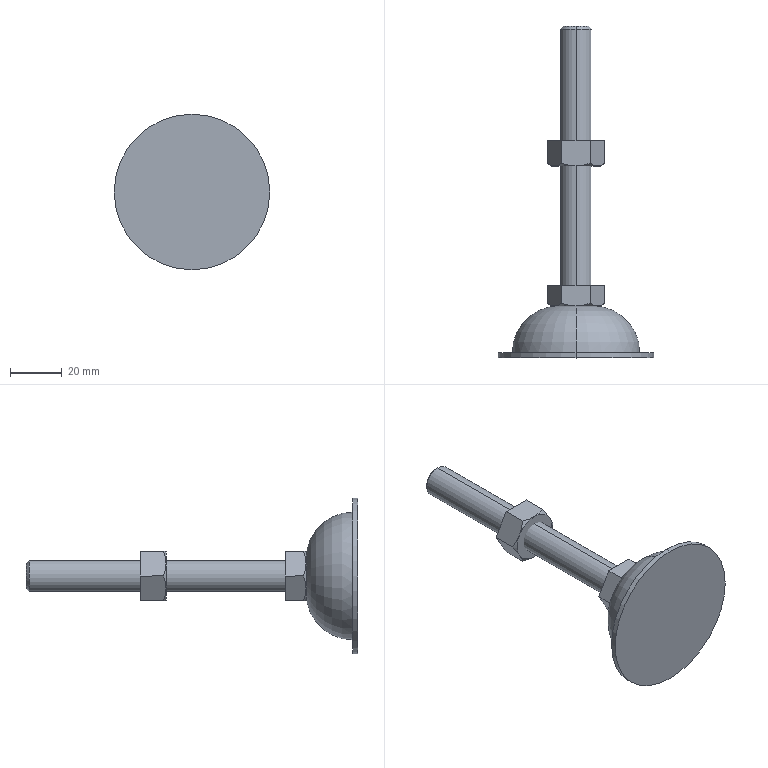Part | SolidWorks | features ICE 4, Chamfer 1, Revolution 1 | 2 solids | 39 faces | box 60 x 128 x 60 mm | volume 47779 mm3 | plane 19 | cone 14 | cylinder 4 | torus 2 | commonest cylinder face diameters 12 x2 60 x2
STEP:
#1=CARTESIAN_POINT('',(0.,28.,6.));
#2=VERTEX_POINT('',#1);
#3=CARTESIAN_POINT('',(0.,28.,-6.));
#4=VERTEX_POINT('',#3);
#5=CARTESIAN_POINT('',(0.,28.,0.));
#6=DIRECTION('',(0.,1.,0.));
#7=DIRECTION('',(0.,0.,1.));
#8=AXIS2_PLACEMENT_3D('',#5,#6,#7);
#9=CIRCLE('',#8,6.);
#10=EDGE_CURVE('',#2,#4,#9,.T.);
#11=ORIENTED_EDGE('',*,*,#10,.T.);
#12=CARTESIAN_POINT('',(0.,126.8,-6.));
#13=VERTEX_POINT('',#12);
#14=CARTESIAN_POINT('',(0.,128.,-6.));
#15=DIRECTION('',(0.,1.,0.));
#16=VECTOR('',#15,1000.);
#17=LINE('',#14,#16);
#18=EDGE_CURVE('',#4,#13,#17,.T.);
#19=ORIENTED_EDGE('',*,*,#18,.T.);
#20=CARTESIAN_POINT('',(0.,126.8,6.));
#21=VERTEX_POINT('',#20);
#22=CARTESIAN_POINT('',(0.,126.8,0.));
#23=DIRECTION('',(0.,-1.,0.));
#24=DIRECTION('',(0.,0.,-1.));
#25=AXIS2_PLACEMENT_3D('',#22,#23,#24);
#26=CIRCLE('',#25,6.);
#27=EDGE_CURVE('',#13,#21,#26,.T.);
#28=ORIENTED_EDGE('',*,*,#27,.T.);
#29=CARTESIAN_POINT('',(0.,128.,6.));
#30=DIRECTION('',(0.,1.,0.));
#31=VECTOR('',#30,1000.);
#32=LINE('',#29,#31);
#33=EDGE_CURVE('',#2,#21,#32,.T.);
#34=ORIENTED_EDGE('',*,*,#33,.F.);
#35=EDGE_LOOP('',(#11,#19,#28,#34));
#36=FACE_OUTER_BOUND('',#35,.T.);
#37=CARTESIAN_POINT('',(0.,128.,0.));
#38=DIRECTION('',(0.,1.,0.));
#39=DIRECTION('',(0.,0.,1.));
#40=AXIS2_PLACEMENT_3D('',#37,#38,#39);
#41=CYLINDRICAL_SURFACE('',#40,6.);
#42=ADVANCED_FACE('',(#36),#41,.T.);
#43=CARTESIAN_POINT('',(0.,128.,4.8));
#44=VERTEX_POINT('',#43);
#45=CARTESIAN_POINT('',(0.,128.,-4.8));
#46=VERTEX_POINT('',#45);
#47=CARTESIAN_POINT('',(0.,128.,0.));
#48=DIRECTION('',(0.,1.,0.));
#49=DIRECTION('',(0.,0.,-1.));
#50=AXIS2_PLACEMENT_3D('',#47,#48,#49);
#51=CIRCLE('',#50,4.8);
#52=EDGE_CURVE('',#44,#46,#51,.T.);
#53=ORIENTED_EDGE('',*,*,#52,.F.);
#54=CARTESIAN_POINT('',(0.,128.,4.8));
#55=DIRECTION('',(0.,-0.7071,0.7071));
#56=VECTOR('',#55,1000.);
#57=LINE('',#54,#56);
#58=EDGE_CURVE('',#44,#21,#57,.T.);
#59=ORIENTED_EDGE('',*,*,#58,.T.);
#60=ORIENTED_EDGE('',*,*,#27,.F.);
#61=CARTESIAN_POINT('',(0.,128.,-4.8));
#62=DIRECTION('',(0.,-0.7071,-0.7071));
#63=VECTOR('',#62,1000.);
#64=LINE('',#61,#63);
#65=EDGE_CURVE('',#46,#13,#64,.T.);
#66=ORIENTED_EDGE('',*,*,#65,.F.);
#67=EDGE_LOOP('',(#53,#59,#60,#66));
#68=FACE_OUTER_BOUND('',#67,.T.);
#69=CARTESIAN_POINT('',(0.,128.,0.));
#70=DIRECTION('',(0.,-1.,0.));
#71=DIRECTION('',(0.,0.,-1.));
#72=AXIS2_PLACEMENT_3D('',#69,#70,#71);
#73=CONICAL_SURFACE('',#72,4.8,0.7854);
#74=ADVANCED_FACE('',(#68),#73,.T.);
#75=CARTESIAN_POINT('',(0.,2.,24.6));
#76=VERTEX_POINT('',#75);
#77=CARTESIAN_POINT('',(0.,2.,-24.6));
#78=VERTEX_POINT('',#77);
#79=CARTESIAN_POINT('',(0.,2.,0.));
#80=DIRECTION('',(0.,1.,0.));
#81=DIRECTION('',(0.,0.,1.));
#82=AXIS2_PLACEMENT_3D('',#79,#80,#81);
#83=CIRCLE('',#82,24.6);
#84=EDGE_CURVE('',#76,#78,#83,.T.);
#85=ORIENTED_EDGE('',*,*,#84,.T.);
#86=CARTESIAN_POINT('',(0.,20.,-6.6));
#87=VERTEX_POINT('',#86);
#88=CARTESIAN_POINT('',(0.,2.,-6.6));
#89=DIRECTION('',(1.,0.,0.));
#90=DIRECTION('',(0.,0.,-1.));
#91=AXIS2_PLACEMENT_3D('',#88,#89,#90);
#92=CIRCLE('',#91,18.);
#93=EDGE_CURVE('',#78,#87,#92,.T.);
#94=ORIENTED_EDGE('',*,*,#93,.T.);
#95=CARTESIAN_POINT('',(0.,20.,6.6));
#96=VERTEX_POINT('',#95);
#97=CARTESIAN_POINT('',(0.,20.,0.));
#98=DIRECTION('',(0.,1.,0.));
#99=DIRECTION('',(0.,0.,1.));
#100=AXIS2_PLACEMENT_3D('',#97,#98,#99);
#101=CIRCLE('',#100,6.6);
#102=EDGE_CURVE('',#96,#87,#101,.T.);
#103=ORIENTED_EDGE('',*,*,#102,.F.);
#104=CARTESIAN_POINT('',(0.,2.,6.6));
#105=DIRECTION('',(-1.,0.,0.));
#106=DIRECTION('',(0.,0.,1.));
#107=AXIS2_PLACEMENT_3D('',#104,#105,#106);
#108=CIRCLE('',#107,18.);
#109=EDGE_CURVE('',#76,#96,#108,.T.);
#110=ORIENTED_EDGE('',*,*,#109,.F.);
#111=EDGE_LOOP('',(#85,#94,#103,#110));
#112=FACE_OUTER_BOUND('',#111,.T.);
#113=CARTESIAN_POINT('',(0.,2.,0.));
#114=DIRECTION('',(0.,1.,0.));
#115=DIRECTION('',(0.,0.,1.));
#116=AXIS2_PLACEMENT_3D('',#113,#114,#115);
#117=TOROIDAL_SURFACE('',#116,6.6,18.);
#118=ADVANCED_FACE('',(#112),#117,.T.);
#119=CARTESIAN_POINT('',(0.,0.,30.));
#120=VERTEX_POINT('',#119);
#121=CARTESIAN_POINT('',(0.,0.,-30.));
#122=VERTEX_POINT('',#121);
#123=CARTESIAN_POINT('',(0.,0.,0.));
#124=DIRECTION('',(0.,1.,0.));
#125=DIRECTION('',(0.,0.,1.));
#126=AXIS2_PLACEMENT_3D('',#123,#124,#125);
#127=CIRCLE('',#126,30.);
#128=EDGE_CURVE('',#120,#122,#127,.T.);
#129=ORIENTED_EDGE('',*,*,#128,.T.);
#130=CARTESIAN_POINT('',(0.,2.,-30.));
#131=VERTEX_POINT('',#130);
#132=CARTESIAN_POINT('',(0.,128.,-30.));
#133=DIRECTION('',(0.,1.,0.));
#134=VECTOR('',#133,1000.);
#135=LINE('',#132,#134);
#136=EDGE_CURVE('',#122,#131,#135,.T.);
#137=ORIENTED_EDGE('',*,*,#136,.T.);
#138=CARTESIAN_POINT('',(0.,2.,30.));
#139=VERTEX_POINT('',#138);
#140=CARTESIAN_POINT('',(0.,2.,0.));
#141=DIRECTION('',(0.,1.,0.));
#142=DIRECTION('',(0.,0.,1.));
#143=AXIS2_PLACEMENT_3D('',#140,#141,#142);
#144=CIRCLE('',#143,30.);
#145=EDGE_CURVE('',#139,#131,#144,.T.);
#146=ORIENTED_EDGE('',*,*,#145,.F.);
#147=CARTESIAN_POINT('',(0.,128.,30.));
#148=DIRECTION('',(0.,1.,0.));
#149=VECTOR('',#148,1000.);
#150=LINE('',#147,#149);
#151=EDGE_CURVE('',#120,#139,#150,.T.);
#152=ORIENTED_EDGE('',*,*,#151,.F.);
#153=EDGE_LOOP('',(#129,#137,#146,#152));
#154=FACE_OUTER_BOUND('',#153,.T.);
#155=CARTESIAN_POINT('',(0.,128.,0.));
#156=DIRECTION('',(0.,1.,0.));
#157=DIRECTION('',(0.,0.,1.));
#158=AXIS2_PLACEMENT_3D('',#155,#156,#157);
#159=CYLINDRICAL_SURFACE('',#158,30.);
#160=ADVANCED_FACE('',(#154),#159,.T.);
#161=ORIENTED_EDGE('',*,*,#102,.T.);
#162=CARTESIAN_POINT('',(0.,20.,0.));
#163=DIRECTION('',(0.,1.,0.));
#164=DIRECTION('',(0.,0.,1.));
#165=AXIS2_PLACEMENT_3D('',#162,#163,#164);
#166=CIRCLE('',#165,6.6);
#167=EDGE_CURVE('',#87,#96,#166,.T.);
#168=ORIENTED_EDGE('',*,*,#167,.T.);
#169=EDGE_LOOP('',(#161,#168));
#170=FACE_BOUND('',#169,.T.);
#171=CARTESIAN_POINT('',(8.227,20.,4.75));
#172=VERTEX_POINT('',#171);
#173=CARTESIAN_POINT('',(0.,20.,9.5));
#174=VERTEX_POINT('',#173);
#175=CARTESIAN_POINT('',(0.,20.,0.));
#176=DIRECTION('',(0.,-1.,0.));
#177=DIRECTION('',(0.,0.,-1.));
#178=AXIS2_PLACEMENT_3D('',#175,#176,#177);
#179=CIRCLE('',#178,9.5);
#180=EDGE_CURVE('',#172,#174,#179,.T.);
#181=ORIENTED_EDGE('',*,*,#180,.T.);
#182=CARTESIAN_POINT('',(-8.227,20.,4.75));
#183=VERTEX_POINT('',#182);
#184=CARTESIAN_POINT('',(0.,20.,0.));
#185=DIRECTION('',(0.,-1.,0.));
#186=DIRECTION('',(0.,0.,-1.));
#187=AXIS2_PLACEMENT_3D('',#184,#185,#186);
#188=CIRCLE('',#187,9.5);
#189=EDGE_CURVE('',#174,#183,#188,.T.);
#190=ORIENTED_EDGE('',*,*,#189,.T.);
#191=CARTESIAN_POINT('',(-8.227,20.,-4.75));
#192=VERTEX_POINT('',#191);
#193=CARTESIAN_POINT('',(0.,20.,0.));
#194=DIRECTION('',(0.,-1.,0.));
#195=DIRECTION('',(0.,0.,-1.));
#196=AXIS2_PLACEMENT_3D('',#193,#194,#195);
#197=CIRCLE('',#196,9.5);
#198=EDGE_CURVE('',#183,#192,#197,.T.);
#199=ORIENTED_EDGE('',*,*,#198,.T.);
#200=CARTESIAN_POINT('',(0.,20.,-9.5));
#201=VERTEX_POINT('',#200);
#202=CARTESIAN_POINT('',(0.,20.,0.));
#203=DIRECTION('',(0.,-1.,0.));
#204=DIRECTION('',(0.,0.,-1.));
#205=AXIS2_PLACEMENT_3D('',#202,#203,#204);
#206=CIRCLE('',#205,9.5);
#207=EDGE_CURVE('',#192,#201,#206,.T.);
#208=ORIENTED_EDGE('',*,*,#207,.T.);
#209=CARTESIAN_POINT('',(8.227,20.,-4.75));
#210=VERTEX_POINT('',#209);
#211=CARTESIAN_POINT('',(0.,20.,0.));
#212=DIRECTION('',(0.,-1.,0.));
#213=DIRECTION('',(0.,0.,-1.));
#214=AXIS2_PLACEMENT_3D('',#211,#212,#213);
#215=CIRCLE('',#214,9.5);
#216=EDGE_CURVE('',#201,#210,#215,.T.);
#217=ORIENTED_EDGE('',*,*,#216,.T.);
#218=CARTESIAN_POINT('',(0.,20.,0.));
#219=DIRECTION('',(0.,-1.,0.));
#220=DIRECTION('',(0.,0.,-1.));
#221=AXIS2_PLACEMENT_3D('',#218,#219,#220);
#222=CIRCLE('',#221,9.5);
#223=EDGE_CURVE('',#210,#172,#222,.T.);
#224=ORIENTED_EDGE('',*,*,#223,.T.);
#225=EDGE_LOOP('',(#181,#190,#199,#208,#217,#224));
#226=FACE_OUTER_BOUND('',#225,.T.);
#227=CARTESIAN_POINT('',(-10.97,20.,0.));
#228=DIRECTION('',(0.,1.,0.));
#229=DIRECTION('',(0.,0.,1.));
#230=AXIS2_PLACEMENT_3D('',#227,#228,#229);
#231=PLANE('',#230);
#232=ADVANCED_FACE('',(#170,#226),#231,.F.);
#233=ORIENTED_EDGE('',*,*,#128,.F.);
#234=CARTESIAN_POINT('',(0.,0.,0.));
#235=DIRECTION('',(0.,1.,0.));
#236=DIRECTION('',(0.,0.,1.));
#237=AXIS2_PLACEMENT_3D('',#234,#235,#236);
#238=CIRCLE('',#237,30.);
#239=EDGE_CURVE('',#122,#120,#238,.T.);
#240=ORIENTED_EDGE('',*,*,#239,.F.);
#241=EDGE_LOOP('',(#233,#240));
#242=FACE_OUTER_BOUND('',#241,.T.);
#243=CARTESIAN_POINT('',(0.,0.,0.));
#244=DIRECTION('',(0.,1.,0.));
#245=DIRECTION('',(0.,0.,1.));
#246=AXIS2_PLACEMENT_3D('',#243,#244,#245);
#247=PLANE('',#246);
#248=ADVANCED_FACE('',(#242),#247,.F.);
#249=ORIENTED_EDGE('',*,*,#136,.F.);
#250=ORIENTED_EDGE('',*,*,#239,.T.);
#251=ORIENTED_EDGE('',*,*,#151,.T.);
#252=CARTESIAN_POINT('',(0.,2.,0.));
#253=DIRECTION('',(0.,1.,0.));
#254=DIRECTION('',(0.,0.,1.));
#255=AXIS2_PLACEMENT_3D('',#252,#253,#254);
#256=CIRCLE('',#255,30.);
#257=EDGE_CURVE('',#131,#139,#256,.T.);
#258=ORIENTED_EDGE('',*,*,#257,.F.);
#259=EDGE_LOOP('',(#249,#250,#251,#258));
#260=FACE_OUTER_BOUND('',#259,.T.);
#261=CARTESIAN_POINT('',(0.,128.,0.));
#262=DIRECTION('',(0.,1.,0.));
#263=DIRECTION('',(0.,0.,1.));
#264=AXIS2_PLACEMENT_3D('',#261,#262,#263);
#265=CYLINDRICAL_SURFACE('',#264,30.);
#266=ADVANCED_FACE('',(#260),#265,.T.);
#267=ORIENTED_EDGE('',*,*,#84,.F.);
#268=CARTESIAN_POINT('',(0.,2.,0.));
#269=DIRECTION('',(0.,1.,0.));
#270=DIRECTION('',(0.,0.,1.));
#271=AXIS2_PLACEMENT_3D('',#268,#269,#270);
#272=CIRCLE('',#271,24.6);
#273=EDGE_CURVE('',#78,#76,#272,.T.);
#274=ORIENTED_EDGE('',*,*,#273,.F.);
#275=EDGE_LOOP('',(#267,#274));
#276=FACE_BOUND('',#275,.T.);
#277=ORIENTED_EDGE('',*,*,#145,.T.);
#278=ORIENTED_EDGE('',*,*,#257,.T.);
#279=EDGE_LOOP('',(#277,#278));
#280=FACE_OUTER_BOUND('',#279,.T.);
#281=CARTESIAN_POINT('',(0.,2.,30.));
#282=DIRECTION('',(0.,-1.,0.));
#283=DIRECTION('',(0.,0.,-1.));
#284=AXIS2_PLACEMENT_3D('',#281,#282,#283);
#285=PLANE('',#284);
#286=ADVANCED_FACE('',(#276,#280),#285,.F.);
#287=ORIENTED_EDGE('',*,*,#93,.F.);
#288=ORIENTED_EDGE('',*,*,#273,.T.);
#289=ORIENTED_EDGE('',*,*,#109,.T.);
#290=ORIENTED_EDGE('',*,*,#167,.F.);
#291=EDGE_LOOP('',(#287,#288,#289,#290));
#292=FACE_OUTER_BOUND('',#291,.T.);
#293=CARTESIAN_POINT('',(0.,2.,0.));
#294=DIRECTION('',(0.,1.,0.));
#295=DIRECTION('',(0.,0.,1.));
#296=AXIS2_PLACEMENT_3D('',#293,#294,#295);
#297=TOROIDAL_SURFACE('',#296,6.6,18.);
#298=ADVANCED_FACE('',(#292),#297,.T.);
#299=CARTESIAN_POINT('',(5.485,21.029,-9.5));
#300=VERTEX_POINT('',#299);
#301=CARTESIAN_POINT('',(5.485,21.029,-9.5));
#302=CARTESIAN_POINT('',(5.93,20.717,-8.729));
#303=CARTESIAN_POINT('',(6.38,20.459,-7.95));
#304=CARTESIAN_POINT('',(7.293,20.1,-6.369));
#305=CARTESIAN_POINT('',(7.756,20.,-5.567));
#306=CARTESIAN_POINT('',(8.227,20.,-4.75));
#307=B_SPLINE_CURVE_WITH_KNOTS('',3,(#301,#302,#303,#304,#305,#306),.UNSPECIFIED.,.F.,.F.,(4,2,4),(0.000000241,0.00279,0.00558),.UNSPECIFIED.);
#308=EDGE_CURVE('',#300,#210,#307,.T.);
#309=ORIENTED_EDGE('',*,*,#308,.T.);
#310=ORIENTED_EDGE('',*,*,#216,.F.);
#311=CARTESIAN_POINT('',(0.,20.,-9.5));
#312=CARTESIAN_POINT('',(0.466,20.,-9.5));
#313=CARTESIAN_POINT('',(0.9352,20.024,-9.5));
#314=CARTESIAN_POINT('',(1.875,20.12,-9.5));
#315=CARTESIAN_POINT('',(2.338,20.192,-9.5));
#316=CARTESIAN_POINT('',(3.711,20.463,-9.5));
#317=CARTESIAN_POINT('',(4.605,20.721,-9.5));
#318=CARTESIAN_POINT('',(5.485,21.029,-9.5));
#319=B_SPLINE_CURVE_WITH_KNOTS('',3,(#311,#312,#313,#314,#315,#316,#317,#318),.UNSPECIFIED.,.F.,.F.,(4,2,2,4),(0.01437,0.01576,0.01716,0.01995),.UNSPECIFIED.);
#320=EDGE_CURVE('',#201,#300,#319,.T.);
#321=ORIENTED_EDGE('',*,*,#320,.T.);
#322=EDGE_LOOP('',(#309,#310,#321));
#323=FACE_OUTER_BOUND('',#322,.T.);
#324=CARTESIAN_POINT('',(0.,20.,0.));
#325=DIRECTION('',(0.,1.,0.));
#326=DIRECTION('',(0.,0.,-1.));
#327=AXIS2_PLACEMENT_3D('',#324,#325,#326);
#328=CONICAL_SURFACE('',#327,9.5,0.9599);
#329=ADVANCED_FACE('',(#323),#328,.T.);
#330=CARTESIAN_POINT('',(-5.485,21.029,-9.5));
#331=VERTEX_POINT('',#330);
#332=CARTESIAN_POINT('',(-8.227,20.,-4.75));
#333=CARTESIAN_POINT('',(-7.993,20.,-5.155));
#334=CARTESIAN_POINT('',(-7.757,20.025,-5.565));
#335=CARTESIAN_POINT('',(-7.292,20.12,-6.371));
#336=CARTESIAN_POINT('',(-7.061,20.191,-6.77));
#337=CARTESIAN_POINT('',(-6.376,20.461,-7.956));
#338=CARTESIAN_POINT('',(-5.928,20.719,-8.733));
#339=CARTESIAN_POINT('',(-5.485,21.029,-9.5));
#340=B_SPLINE_CURVE_WITH_KNOTS('',3,(#332,#333,#334,#335,#336,#337,#338,#339),.UNSPECIFIED.,.F.,.F.,(4,2,2,4),(0.00558,0.006964,0.008349,0.01112),.UNSPECIFIED.);
#341=EDGE_CURVE('',#192,#331,#340,.T.);
#342=ORIENTED_EDGE('',*,*,#341,.T.);
#343=CARTESIAN_POINT('',(-5.485,21.029,-9.5));
#344=CARTESIAN_POINT('',(-4.602,20.72,-9.5));
#345=CARTESIAN_POINT('',(-3.69,20.458,-9.5));
#346=CARTESIAN_POINT('',(-1.858,20.098,-9.5));
#347=CARTESIAN_POINT('',(-0.9336,20.,-9.5));
#348=CARTESIAN_POINT('',(0.,20.,-9.5));
#349=B_SPLINE_CURVE_WITH_KNOTS('',3,(#343,#344,#345,#346,#347,#348),.UNSPECIFIED.,.F.,.F.,(4,2,4),(0.008777,0.01157,0.01437),.UNSPECIFIED.);
#350=EDGE_CURVE('',#331,#201,#349,.T.);
#351=ORIENTED_EDGE('',*,*,#350,.T.);
#352=ORIENTED_EDGE('',*,*,#207,.F.);
#353=EDGE_LOOP('',(#342,#351,#352));
#354=FACE_OUTER_BOUND('',#353,.T.);
#355=CARTESIAN_POINT('',(0.,20.,0.));
#356=DIRECTION('',(0.,1.,0.));
#357=DIRECTION('',(0.,0.,-1.));
#358=AXIS2_PLACEMENT_3D('',#355,#356,#357);
#359=CONICAL_SURFACE('',#358,9.5,0.9599);
#360=ADVANCED_FACE('',(#354),#359,.T.);
#361=CARTESIAN_POINT('',(10.97,21.029,0.));
#362=VERTEX_POINT('',#361);
#363=CARTESIAN_POINT('',(10.97,21.029,0.));
#364=CARTESIAN_POINT('',(10.524,20.717,0.7712));
#365=CARTESIAN_POINT('',(10.075,20.459,1.55));
#366=CARTESIAN_POINT('',(9.162,20.1,3.131));
#367=CARTESIAN_POINT('',(8.699,20.,3.933));
#368=CARTESIAN_POINT('',(8.227,20.,4.75));
#369=B_SPLINE_CURVE_WITH_KNOTS('',3,(#363,#364,#365,#366,#367,#368),.UNSPECIFIED.,.F.,.F.,(4,2,4),(0.000000241,0.00279,0.00558),.UNSPECIFIED.);
#370=EDGE_CURVE('',#362,#172,#369,.T.);
#371=ORIENTED_EDGE('',*,*,#370,.T.);
#372=ORIENTED_EDGE('',*,*,#223,.F.);
#373=CARTESIAN_POINT('',(8.227,20.,-4.75));
#374=CARTESIAN_POINT('',(8.461,20.,-4.345));
#375=CARTESIAN_POINT('',(8.698,20.025,-3.935));
#376=CARTESIAN_POINT('',(9.163,20.12,-3.129));
#377=CARTESIAN_POINT('',(9.393,20.191,-2.73));
#378=CARTESIAN_POINT('',(10.078,20.461,-1.544));
#379=CARTESIAN_POINT('',(10.527,20.719,-0.7675));
#380=CARTESIAN_POINT('',(10.97,21.029,0.));
#381=B_SPLINE_CURVE_WITH_KNOTS('',3,(#373,#374,#375,#376,#377,#378,#379,#380),.UNSPECIFIED.,.F.,.F.,(4,2,2,4),(0.00558,0.006964,0.008349,0.01112),.UNSPECIFIED.);
#382=EDGE_CURVE('',#210,#362,#381,.T.);
#383=ORIENTED_EDGE('',*,*,#382,.T.);
#384=EDGE_LOOP('',(#371,#372,#383));
#385=FACE_OUTER_BOUND('',#384,.T.);
#386=CARTESIAN_POINT('',(0.,20.,0.));
#387=DIRECTION('',(0.,1.,0.));
#388=DIRECTION('',(0.,0.,-1.));
#389=AXIS2_PLACEMENT_3D('',#386,#387,#388);
#390=CONICAL_SURFACE('',#389,9.5,0.9599);
#391=ADVANCED_FACE('',(#385),#390,.T.);
#392=CARTESIAN_POINT('',(5.485,21.029,9.5));
#393=VERTEX_POINT('',#392);
#394=CARTESIAN_POINT('',(5.485,21.029,9.5));
#395=CARTESIAN_POINT('',(4.605,20.721,9.5));
#396=CARTESIAN_POINT('',(3.711,20.463,9.5));
#397=CARTESIAN_POINT('',(2.338,20.192,9.5));
#398=CARTESIAN_POINT('',(1.875,20.12,9.5));
#399=CARTESIAN_POINT('',(0.9352,20.024,9.5));
#400=CARTESIAN_POINT('',(0.466,20.,9.5));
#401=CARTESIAN_POINT('',(0.,20.,9.5));
#402=B_SPLINE_CURVE_WITH_KNOTS('',3,(#394,#395,#396,#397,#398,#399,#400,#401),.UNSPECIFIED.,.F.,.F.,(4,2,2,4),(0.02216,0.02495,0.02635,0.02774),.UNSPECIFIED.);
#403=EDGE_CURVE('',#393,#174,#402,.T.);
#404=ORIENTED_EDGE('',*,*,#403,.T.);
#405=ORIENTED_EDGE('',*,*,#180,.F.);
#406=CARTESIAN_POINT('',(8.227,20.,4.75));
#407=CARTESIAN_POINT('',(7.993,20.,5.155));
#408=CARTESIAN_POINT('',(7.757,20.025,5.565));
#409=CARTESIAN_POINT('',(7.292,20.12,6.371));
#410=CARTESIAN_POINT('',(7.061,20.191,6.77));
#411=CARTESIAN_POINT('',(6.376,20.461,7.956));
#412=CARTESIAN_POINT('',(5.928,20.719,8.733));
#413=CARTESIAN_POINT('',(5.485,21.029,9.5));
#414=B_SPLINE_CURVE_WITH_KNOTS('',3,(#406,#407,#408,#409,#410,#411,#412,#413),.UNSPECIFIED.,.F.,.F.,(4,2,2,4),(0.00558,0.006964,0.008349,0.01112),.UNSPECIFIED.);
#415=EDGE_CURVE('',#172,#393,#414,.T.);
#416=ORIENTED_EDGE('',*,*,#415,.T.);
#417=EDGE_LOOP('',(#404,#405,#416));
#418=FACE_OUTER_BOUND('',#417,.T.);
#419=CARTESIAN_POINT('',(0.,20.,0.));
#420=DIRECTION('',(0.,1.,0.));
#421=DIRECTION('',(0.,0.,-1.));
#422=AXIS2_PLACEMENT_3D('',#419,#420,#421);
#423=CONICAL_SURFACE('',#422,9.5,0.9599);
#424=ADVANCED_FACE('',(#418),#423,.T.);
#425=CARTESIAN_POINT('',(-5.485,21.029,9.5));
#426=VERTEX_POINT('',#425);
#427=CARTESIAN_POINT('',(0.,20.,9.5));
#428=CARTESIAN_POINT('',(-0.9336,20.,9.5));
#429=CARTESIAN_POINT('',(-1.858,20.098,9.5));
#430=CARTESIAN_POINT('',(-3.69,20.458,9.5));
#431=CARTESIAN_POINT('',(-4.602,20.72,9.5));
#432=CARTESIAN_POINT('',(-5.485,21.029,9.5));
#433=B_SPLINE_CURVE_WITH_KNOTS('',3,(#427,#428,#429,#430,#431,#432),.UNSPECIFIED.,.F.,.F.,(4,2,4),(0.02774,0.03054,0.03334),.UNSPECIFIED.);
#434=EDGE_CURVE('',#174,#426,#433,.T.);
#435=ORIENTED_EDGE('',*,*,#434,.T.);
#436=CARTESIAN_POINT('',(-5.485,21.029,9.5));
#437=CARTESIAN_POINT('',(-5.93,20.717,8.729));
#438=CARTESIAN_POINT('',(-6.38,20.459,7.95));
#439=CARTESIAN_POINT('',(-7.293,20.1,6.369));
#440=CARTESIAN_POINT('',(-7.756,20.,5.567));
#441=CARTESIAN_POINT('',(-8.227,20.,4.75));
#442=B_SPLINE_CURVE_WITH_KNOTS('',3,(#436,#437,#438,#439,#440,#441),.UNSPECIFIED.,.F.,.F.,(4,2,4),(0.000000241,0.00279,0.00558),.UNSPECIFIED.);
#443=EDGE_CURVE('',#426,#183,#442,.T.);
#444=ORIENTED_EDGE('',*,*,#443,.T.);
#445=ORIENTED_EDGE('',*,*,#189,.F.);
#446=EDGE_LOOP('',(#435,#444,#445));
#447=FACE_OUTER_BOUND('',#446,.T.);
#448=CARTESIAN_POINT('',(0.,20.,0.));
#449=DIRECTION('',(0.,1.,0.));
#450=DIRECTION('',(0.,0.,-1.));
#451=AXIS2_PLACEMENT_3D('',#448,#449,#450);
#452=CONICAL_SURFACE('',#451,9.5,0.9599);
#453=ADVANCED_FACE('',(#447),#452,.T.);
#454=CARTESIAN_POINT('',(-10.97,21.029,0.));
#455=VERTEX_POINT('',#454);
#456=CARTESIAN_POINT('',(-8.227,20.,4.75));
#457=CARTESIAN_POINT('',(-8.461,20.,4.345));
#458=CARTESIAN_POINT('',(-8.698,20.025,3.935));
#459=CARTESIAN_POINT('',(-9.163,20.12,3.129));
#460=CARTESIAN_POINT('',(-9.393,20.191,2.73));
#461=CARTESIAN_POINT('',(-10.078,20.461,1.544));
#462=CARTESIAN_POINT('',(-10.527,20.719,0.7675));
#463=CARTESIAN_POINT('',(-10.97,21.029,0.));
#464=B_SPLINE_CURVE_WITH_KNOTS('',3,(#456,#457,#458,#459,#460,#461,#462,#463),.UNSPECIFIED.,.F.,.F.,(4,2,2,4),(0.00558,0.006964,0.008349,0.01112),.UNSPECIFIED.);
#465=EDGE_CURVE('',#183,#455,#464,.T.);
#466=ORIENTED_EDGE('',*,*,#465,.T.);
#467=CARTESIAN_POINT('',(-10.97,21.029,0.));
#468=CARTESIAN_POINT('',(-10.524,20.717,-0.7712));
#469=CARTESIAN_POINT('',(-10.075,20.459,-1.55));
#470=CARTESIAN_POINT('',(-9.162,20.1,-3.131));
#471=CARTESIAN_POINT('',(-8.699,20.,-3.933));
#472=CARTESIAN_POINT('',(-8.227,20.,-4.75));
#473=B_SPLINE_CURVE_WITH_KNOTS('',3,(#467,#468,#469,#470,#471,#472),.UNSPECIFIED.,.F.,.F.,(4,2,4),(0.000000241,0.00279,0.00558),.UNSPECIFIED.);
#474=EDGE_CURVE('',#455,#192,#473,.T.);
#475=ORIENTED_EDGE('',*,*,#474,.T.);
#476=ORIENTED_EDGE('',*,*,#198,.F.);
#477=EDGE_LOOP('',(#466,#475,#476));
#478=FACE_OUTER_BOUND('',#477,.T.);
#479=CARTESIAN_POINT('',(0.,20.,0.));
#480=DIRECTION('',(0.,1.,0.));
#481=DIRECTION('',(0.,0.,-1.));
#482=AXIS2_PLACEMENT_3D('',#479,#480,#481);
#483=CONICAL_SURFACE('',#482,9.5,0.9599);
#484=ADVANCED_FACE('',(#478),#483,.T.);
#485=CARTESIAN_POINT('',(0.,128.,0.));
#486=DIRECTION('',(0.,1.,0.));
#487=DIRECTION('',(0.,0.,-1.));
#488=AXIS2_PLACEMENT_3D('',#485,#486,#487);
#489=CIRCLE('',#488,4.8);
#490=EDGE_CURVE('',#46,#44,#489,.T.);
#491=ORIENTED_EDGE('',*,*,#490,.T.);
#492=ORIENTED_EDGE('',*,*,#52,.T.);
#493=EDGE_LOOP('',(#491,#492));
#494=FACE_OUTER_BOUND('',#493,.T.);
#495=CARTESIAN_POINT('',(0.,128.,0.));
#496=DIRECTION('',(0.,-1.,0.));
#497=DIRECTION('',(0.,0.,-1.));
#498=AXIS2_PLACEMENT_3D('',#495,#496,#497);
#499=PLANE('',#498);
#500=ADVANCED_FACE('',(#494),#499,.F.);
#501=ORIENTED_EDGE('',*,*,#58,.F.);
#502=ORIENTED_EDGE('',*,*,#490,.F.);
#503=ORIENTED_EDGE('',*,*,#65,.T.);
#504=CARTESIAN_POINT('',(0.,126.8,0.));
#505=DIRECTION('',(0.,-1.,0.));
#506=DIRECTION('',(0.,0.,-1.));
#507=AXIS2_PLACEMENT_3D('',#504,#505,#506);
#508=CIRCLE('',#507,6.);
#509=EDGE_CURVE('',#21,#13,#508,.T.);
#510=ORIENTED_EDGE('',*,*,#509,.F.);
#511=EDGE_LOOP('',(#501,#502,#503,#510));
#512=FACE_OUTER_BOUND('',#511,.T.);
#513=CARTESIAN_POINT('',(0.,128.,0.));
#514=DIRECTION('',(0.,-1.,0.));
#515=DIRECTION('',(0.,0.,-1.));
#516=AXIS2_PLACEMENT_3D('',#513,#514,#515);
#517=CONICAL_SURFACE('',#516,4.8,0.7854);
#518=ADVANCED_FACE('',(#512),#517,.T.);
#519=ORIENTED_EDGE('',*,*,#18,.F.);
#520=CARTESIAN_POINT('',(0.,28.,0.));
#521=DIRECTION('',(0.,1.,0.));
#522=DIRECTION('',(0.,0.,1.));
#523=AXIS2_PLACEMENT_3D('',#520,#521,#522);
#524=CIRCLE('',#523,6.);
#525=EDGE_CURVE('',#4,#2,#524,.T.);
#526=ORIENTED_EDGE('',*,*,#525,.T.);
#527=ORIENTED_EDGE('',*,*,#33,.T.);
#528=ORIENTED_EDGE('',*,*,#509,.T.);
#529=EDGE_LOOP('',(#519,#526,#527,#528));
#530=FACE_OUTER_BOUND('',#529,.T.);
#531=CARTESIAN_POINT('',(0.,128.,0.));
#532=DIRECTION('',(0.,1.,0.));
#533=DIRECTION('',(0.,0.,1.));
#534=AXIS2_PLACEMENT_3D('',#531,#532,#533);
#535=CYLINDRICAL_SURFACE('',#534,6.);
#536=ADVANCED_FACE('',(#530),#535,.T.);
#537=CARTESIAN_POINT('',(-5.485,28.,-9.5));
#538=VERTEX_POINT('',#537);
#539=CARTESIAN_POINT('',(-10.97,28.,0.));
#540=VERTEX_POINT('',#539);
#541=CARTESIAN_POINT('',(-5.485,28.,-9.5));
#542=DIRECTION('',(-0.5,0.,0.866));
#543=VECTOR('',#542,1000.);
#544=LINE('',#541,#543);
#545=EDGE_CURVE('',#538,#540,#544,.T.);
#546=ORIENTED_EDGE('',*,*,#545,.T.);
#547=CARTESIAN_POINT('',(-5.485,28.,9.5));
#548=VERTEX_POINT('',#547);
#549=CARTESIAN_POINT('',(-10.97,28.,0.));
#550=DIRECTION('',(0.5,0.,0.866));
#551=VECTOR('',#550,1000.);
#552=LINE('',#549,#551);
#553=EDGE_CURVE('',#540,#548,#552,.T.);
#554=ORIENTED_EDGE('',*,*,#553,.T.);
#555=CARTESIAN_POINT('',(5.485,28.,9.5));
#556=VERTEX_POINT('',#555);
#557=CARTESIAN_POINT('',(-5.485,28.,9.5));
#558=DIRECTION('',(1.,0.,0.));
#559=VECTOR('',#558,1000.);
#560=LINE('',#557,#559);
#561=EDGE_CURVE('',#548,#556,#560,.T.);
#562=ORIENTED_EDGE('',*,*,#561,.T.);
#563=CARTESIAN_POINT('',(10.97,28.,0.));
#564=VERTEX_POINT('',#563);
#565=CARTESIAN_POINT('',(5.485,28.,9.5));
#566=DIRECTION('',(0.5,0.,-0.866));
#567=VECTOR('',#566,1000.);
#568=LINE('',#565,#567);
#569=EDGE_CURVE('',#556,#564,#568,.T.);
#570=ORIENTED_EDGE('',*,*,#569,.T.);
#571=CARTESIAN_POINT('',(5.485,28.,-9.5));
#572=VERTEX_POINT('',#571);
#573=CARTESIAN_POINT('',(10.97,28.,0.));
#574=DIRECTION('',(-0.5,0.,-0.866));
#575=VECTOR('',#574,1000.);
#576=LINE('',#573,#575);
#577=EDGE_CURVE('',#564,#572,#576,.T.);
#578=ORIENTED_EDGE('',*,*,#577,.T.);
#579=CARTESIAN_POINT('',(5.485,28.,-9.5));
#580=DIRECTION('',(-1.,0.,0.));
#581=VECTOR('',#580,1000.);
#582=LINE('',#579,#581);
#583=EDGE_CURVE('',#572,#538,#582,.T.);
#584=ORIENTED_EDGE('',*,*,#583,.T.);
#585=EDGE_LOOP('',(#546,#554,#562,#570,#578,#584));
#586=FACE_OUTER_BOUND('',#585,.T.);
#587=ORIENTED_EDGE('',*,*,#10,.F.);
#588=ORIENTED_EDGE('',*,*,#525,.F.);
#589=EDGE_LOOP('',(#587,#588));
#590=FACE_BOUND('',#589,.T.);
#591=CARTESIAN_POINT('',(-10.97,28.,0.));
#592=DIRECTION('',(0.,1.,0.));
#593=DIRECTION('',(0.,0.,1.));
#594=AXIS2_PLACEMENT_3D('',#591,#592,#593);
#595=PLANE('',#594);
#596=ADVANCED_FACE('',(#586,#590),#595,.T.);
#597=ORIENTED_EDGE('',*,*,#350,.F.);
#598=CARTESIAN_POINT('',(-5.485,28.,-9.5));
#599=DIRECTION('',(0.,-1.,0.));
#600=VECTOR('',#599,1000.);
#601=LINE('',#598,#600);
#602=EDGE_CURVE('',#538,#331,#601,.T.);
#603=ORIENTED_EDGE('',*,*,#602,.F.);
#604=ORIENTED_EDGE('',*,*,#583,.F.);
#605=CARTESIAN_POINT('',(5.485,28.,-9.5));
#606=DIRECTION('',(0.,-1.,0.));
#607=VECTOR('',#606,1000.);
#608=LINE('',#605,#607);
#609=EDGE_CURVE('',#572,#300,#608,.T.);
#610=ORIENTED_EDGE('',*,*,#609,.T.);
#611=ORIENTED_EDGE('',*,*,#320,.F.);
#612=EDGE_LOOP('',(#597,#603,#604,#610,#611));
#613=FACE_OUTER_BOUND('',#612,.T.);
#614=CARTESIAN_POINT('',(5.485,28.,-9.5));
#615=DIRECTION('',(0.,0.,1.));
#616=DIRECTION('',(1.,0.,0.));
#617=AXIS2_PLACEMENT_3D('',#614,#615,#616);
#618=PLANE('',#617);
#619=ADVANCED_FACE('',(#613),#618,.F.);
#620=ORIENTED_EDGE('',*,*,#308,.F.);
#621=ORIENTED_EDGE('',*,*,#609,.F.);
#622=ORIENTED_EDGE('',*,*,#577,.F.);
#623=CARTESIAN_POINT('',(10.97,28.,0.));
#624=DIRECTION('',(0.,-1.,0.));
#625=VECTOR('',#624,1000.);
#626=LINE('',#623,#625);
#627=EDGE_CURVE('',#564,#362,#626,.T.);
#628=ORIENTED_EDGE('',*,*,#627,.T.);
#629=ORIENTED_EDGE('',*,*,#382,.F.);
#630=EDGE_LOOP('',(#620,#621,#622,#628,#629));
#631=FACE_OUTER_BOUND('',#630,.T.);
#632=CARTESIAN_POINT('',(10.97,28.,0.));
#633=DIRECTION('',(-0.866,0.,0.5));
#634=DIRECTION('',(0.5,0.,0.866));
#635=AXIS2_PLACEMENT_3D('',#632,#633,#634);
#636=PLANE('',#635);
#637=ADVANCED_FACE('',(#631),#636,.F.);
#638=ORIENTED_EDGE('',*,*,#370,.F.);
#639=ORIENTED_EDGE('',*,*,#627,.F.);
#640=ORIENTED_EDGE('',*,*,#569,.F.);
#641=CARTESIAN_POINT('',(5.485,28.,9.5));
#642=DIRECTION('',(0.,-1.,0.));
#643=VECTOR('',#642,1000.);
#644=LINE('',#641,#643);
#645=EDGE_CURVE('',#556,#393,#644,.T.);
#646=ORIENTED_EDGE('',*,*,#645,.T.);
#647=ORIENTED_EDGE('',*,*,#415,.F.);
#648=EDGE_LOOP('',(#638,#639,#640,#646,#647));
#649=FACE_OUTER_BOUND('',#648,.T.);
#650=CARTESIAN_POINT('',(5.485,28.,9.5));
#651=DIRECTION('',(-0.866,0.,-0.5));
#652=DIRECTION('',(-0.5,0.,0.866));
#653=AXIS2_PLACEMENT_3D('',#650,#651,#652);
#654=PLANE('',#653);
#655=ADVANCED_FACE('',(#649),#654,.F.);
#656=ORIENTED_EDGE('',*,*,#403,.F.);
#657=ORIENTED_EDGE('',*,*,#645,.F.);
#658=ORIENTED_EDGE('',*,*,#561,.F.);
#659=CARTESIAN_POINT('',(-5.485,28.,9.5));
#660=DIRECTION('',(0.,-1.,0.));
#661=VECTOR('',#660,1000.);
#662=LINE('',#659,#661);
#663=EDGE_CURVE('',#548,#426,#662,.T.);
#664=ORIENTED_EDGE('',*,*,#663,.T.);
#665=ORIENTED_EDGE('',*,*,#434,.F.);
#666=EDGE_LOOP('',(#656,#657,#658,#664,#665));
#667=FACE_OUTER_BOUND('',#666,.T.);
#668=CARTESIAN_POINT('',(-5.485,28.,9.5));
#669=DIRECTION('',(0.,0.,-1.));
#670=DIRECTION('',(-1.,0.,0.));
#671=AXIS2_PLACEMENT_3D('',#668,#669,#670);
#672=PLANE('',#671);
#673=ADVANCED_FACE('',(#667),#672,.F.);
#674=ORIENTED_EDGE('',*,*,#443,.F.);
#675=ORIENTED_EDGE('',*,*,#663,.F.);
#676=ORIENTED_EDGE('',*,*,#553,.F.);
#677=CARTESIAN_POINT('',(-10.97,28.,0.));
#678=DIRECTION('',(0.,-1.,0.));
#679=VECTOR('',#678,1000.);
#680=LINE('',#677,#679);
#681=EDGE_CURVE('',#540,#455,#680,.T.);
#682=ORIENTED_EDGE('',*,*,#681,.T.);
#683=ORIENTED_EDGE('',*,*,#465,.F.);
#684=EDGE_LOOP('',(#674,#675,#676,#682,#683));
#685=FACE_OUTER_BOUND('',#684,.T.);
#686=CARTESIAN_POINT('',(-10.97,28.,0.));
#687=DIRECTION('',(0.866,0.,-0.5));
#688=DIRECTION('',(-0.5,0.,-0.866));
#689=AXIS2_PLACEMENT_3D('',#686,#687,#688);
#690=PLANE('',#689);
#691=ADVANCED_FACE('',(#685),#690,.F.);
#692=ORIENTED_EDGE('',*,*,#474,.F.);
#693=ORIENTED_EDGE('',*,*,#681,.F.);
#694=ORIENTED_EDGE('',*,*,#545,.F.);
#695=ORIENTED_EDGE('',*,*,#602,.T.);
#696=ORIENTED_EDGE('',*,*,#341,.F.);
#697=EDGE_LOOP('',(#692,#693,#694,#695,#696));
#698=FACE_OUTER_BOUND('',#697,.T.);
#699=CARTESIAN_POINT('',(-5.485,28.,-9.5));
#700=DIRECTION('',(0.866,0.,0.5));
#701=DIRECTION('',(0.5,0.,-0.866));
#702=AXIS2_PLACEMENT_3D('',#699,#700,#701);
#703=PLANE('',#702);
#704=ADVANCED_FACE('',(#698),#703,.F.);
#705=CLOSED_SHELL('',(#42,#74,#118,#160,#232,#248,#266,#286,#298,#329,#360,#391,#424,#453,#484,#500,#518,#536,#596,#619,#637,#655,#673,#691,#704));
#706=MANIFOLD_SOLID_BREP('',#705);
#707=CARTESIAN_POINT('',(-5.485,75.029,-9.5));
#708=VERTEX_POINT('',#707);
#709=CARTESIAN_POINT('',(0.,74.,-9.5));
#710=VERTEX_POINT('',#709);
#711=CARTESIAN_POINT('',(-5.485,75.029,-9.5));
#712=CARTESIAN_POINT('',(-4.602,74.72,-9.5));
#713=CARTESIAN_POINT('',(-3.69,74.458,-9.5));
#714=CARTESIAN_POINT('',(-1.858,74.098,-9.5));
#715=CARTESIAN_POINT('',(-0.9336,74.,-9.5));
#716=CARTESIAN_POINT('',(0.,74.,-9.5));
#717=B_SPLINE_CURVE_WITH_KNOTS('',3,(#711,#712,#713,#714,#715,#716),.UNSPECIFIED.,.F.,.F.,(4,2,4),(0.008777,0.01157,0.01437),.UNSPECIFIED.);
#718=EDGE_CURVE('',#708,#710,#717,.T.);
#719=ORIENTED_EDGE('',*,*,#718,.F.);
#720=CARTESIAN_POINT('',(-5.485,84.,-9.5));
#721=VERTEX_POINT('',#720);
#722=CARTESIAN_POINT('',(-5.485,84.,-9.5));
#723=DIRECTION('',(0.,-1.,0.));
#724=VECTOR('',#723,1000.);
#725=LINE('',#722,#724);
#726=EDGE_CURVE('',#721,#708,#725,.T.);
#727=ORIENTED_EDGE('',*,*,#726,.F.);
#728=CARTESIAN_POINT('',(5.485,84.,-9.5));
#729=VERTEX_POINT('',#728);
#730=CARTESIAN_POINT('',(5.485,84.,-9.5));
#731=DIRECTION('',(-1.,0.,0.));
#732=VECTOR('',#731,1000.);
#733=LINE('',#730,#732);
#734=EDGE_CURVE('',#729,#721,#733,.T.);
#735=ORIENTED_EDGE('',*,*,#734,.F.);
#736=CARTESIAN_POINT('',(5.485,75.029,-9.5));
#737=VERTEX_POINT('',#736);
#738=CARTESIAN_POINT('',(5.485,84.,-9.5));
#739=DIRECTION('',(0.,-1.,0.));
#740=VECTOR('',#739,1000.);
#741=LINE('',#738,#740);
#742=EDGE_CURVE('',#729,#737,#741,.T.);
#743=ORIENTED_EDGE('',*,*,#742,.T.);
#744=CARTESIAN_POINT('',(0.,74.,-9.5));
#745=CARTESIAN_POINT('',(0.466,74.,-9.5));
#746=CARTESIAN_POINT('',(0.9352,74.024,-9.5));
#747=CARTESIAN_POINT('',(1.875,74.12,-9.5));
#748=CARTESIAN_POINT('',(2.338,74.192,-9.5));
#749=CARTESIAN_POINT('',(3.711,74.463,-9.5));
#750=CARTESIAN_POINT('',(4.605,74.721,-9.5));
#751=CARTESIAN_POINT('',(5.485,75.029,-9.5));
#752=B_SPLINE_CURVE_WITH_KNOTS('',3,(#744,#745,#746,#747,#748,#749,#750,#751),.UNSPECIFIED.,.F.,.F.,(4,2,2,4),(0.01437,0.01576,0.01716,0.01995),.UNSPECIFIED.);
#753=EDGE_CURVE('',#710,#737,#752,.T.);
#754=ORIENTED_EDGE('',*,*,#753,.F.);
#755=EDGE_LOOP('',(#719,#727,#735,#743,#754));
#756=FACE_OUTER_BOUND('',#755,.T.);
#757=CARTESIAN_POINT('',(5.485,84.,-9.5));
#758=DIRECTION('',(0.,0.,1.));
#759=DIRECTION('',(1.,0.,0.));
#760=AXIS2_PLACEMENT_3D('',#757,#758,#759);
#761=PLANE('',#760);
#762=ADVANCED_FACE('',(#756),#761,.F.);
#763=CARTESIAN_POINT('',(-10.97,75.029,0.));
#764=VERTEX_POINT('',#763);
#765=CARTESIAN_POINT('',(-8.227,74.,-4.75));
#766=VERTEX_POINT('',#765);
#767=CARTESIAN_POINT('',(-10.97,75.029,0.));
#768=CARTESIAN_POINT('',(-10.524,74.717,-0.7712));
#769=CARTESIAN_POINT('',(-10.075,74.459,-1.55));
#770=CARTESIAN_POINT('',(-9.162,74.1,-3.131));
#771=CARTESIAN_POINT('',(-8.699,74.,-3.933));
#772=CARTESIAN_POINT('',(-8.227,74.,-4.75));
#773=B_SPLINE_CURVE_WITH_KNOTS('',3,(#767,#768,#769,#770,#771,#772),.UNSPECIFIED.,.F.,.F.,(4,2,4),(0.000000241,0.00279,0.00558),.UNSPECIFIED.);
#774=EDGE_CURVE('',#764,#766,#773,.T.);
#775=ORIENTED_EDGE('',*,*,#774,.F.);
#776=CARTESIAN_POINT('',(-10.97,84.,0.));
#777=VERTEX_POINT('',#776);
#778=CARTESIAN_POINT('',(-10.97,84.,0.));
#779=DIRECTION('',(0.,-1.,0.));
#780=VECTOR('',#779,1000.);
#781=LINE('',#778,#780);
#782=EDGE_CURVE('',#777,#764,#781,.T.);
#783=ORIENTED_EDGE('',*,*,#782,.F.);
#784=CARTESIAN_POINT('',(-5.485,84.,-9.5));
#785=DIRECTION('',(-0.5,0.,0.866));
#786=VECTOR('',#785,1000.);
#787=LINE('',#784,#786);
#788=EDGE_CURVE('',#721,#777,#787,.T.);
#789=ORIENTED_EDGE('',*,*,#788,.F.);
#790=ORIENTED_EDGE('',*,*,#726,.T.);
#791=CARTESIAN_POINT('',(-8.227,74.,-4.75));
#792=CARTESIAN_POINT('',(-7.993,74.,-5.155));
#793=CARTESIAN_POINT('',(-7.757,74.025,-5.565));
#794=CARTESIAN_POINT('',(-7.292,74.12,-6.371));
#795=CARTESIAN_POINT('',(-7.061,74.191,-6.77));
#796=CARTESIAN_POINT('',(-6.376,74.461,-7.956));
#797=CARTESIAN_POINT('',(-5.928,74.719,-8.733));
#798=CARTESIAN_POINT('',(-5.485,75.029,-9.5));
#799=B_SPLINE_CURVE_WITH_KNOTS('',3,(#791,#792,#793,#794,#795,#796,#797,#798),.UNSPECIFIED.,.F.,.F.,(4,2,2,4),(0.00558,0.006964,0.008349,0.01112),.UNSPECIFIED.);
#800=EDGE_CURVE('',#766,#708,#799,.T.);
#801=ORIENTED_EDGE('',*,*,#800,.F.);
#802=EDGE_LOOP('',(#775,#783,#789,#790,#801));
#803=FACE_OUTER_BOUND('',#802,.T.);
#804=CARTESIAN_POINT('',(-5.485,84.,-9.5));
#805=DIRECTION('',(0.866,0.,0.5));
#806=DIRECTION('',(0.5,0.,-0.866));
#807=AXIS2_PLACEMENT_3D('',#804,#805,#806);
#808=PLANE('',#807);
#809=ADVANCED_FACE('',(#803),#808,.F.);
#810=CARTESIAN_POINT('',(-5.485,75.029,9.5));
#811=VERTEX_POINT('',#810);
#812=CARTESIAN_POINT('',(-8.227,74.,4.75));
#813=VERTEX_POINT('',#812);
#814=CARTESIAN_POINT('',(-5.485,75.029,9.5));
#815=CARTESIAN_POINT('',(-5.93,74.717,8.729));
#816=CARTESIAN_POINT('',(-6.38,74.459,7.95));
#817=CARTESIAN_POINT('',(-7.293,74.1,6.369));
#818=CARTESIAN_POINT('',(-7.756,74.,5.567));
#819=CARTESIAN_POINT('',(-8.227,74.,4.75));
#820=B_SPLINE_CURVE_WITH_KNOTS('',3,(#814,#815,#816,#817,#818,#819),.UNSPECIFIED.,.F.,.F.,(4,2,4),(0.000000241,0.00279,0.00558),.UNSPECIFIED.);
#821=EDGE_CURVE('',#811,#813,#820,.T.);
#822=ORIENTED_EDGE('',*,*,#821,.F.);
#823=CARTESIAN_POINT('',(-5.485,84.,9.5));
#824=VERTEX_POINT('',#823);
#825=CARTESIAN_POINT('',(-5.485,84.,9.5));
#826=DIRECTION('',(0.,-1.,0.));
#827=VECTOR('',#826,1000.);
#828=LINE('',#825,#827);
#829=EDGE_CURVE('',#824,#811,#828,.T.);
#830=ORIENTED_EDGE('',*,*,#829,.F.);
#831=CARTESIAN_POINT('',(-10.97,84.,0.));
#832=DIRECTION('',(0.5,0.,0.866));
#833=VECTOR('',#832,1000.);
#834=LINE('',#831,#833);
#835=EDGE_CURVE('',#777,#824,#834,.T.);
#836=ORIENTED_EDGE('',*,*,#835,.F.);
#837=ORIENTED_EDGE('',*,*,#782,.T.);
#838=CARTESIAN_POINT('',(-8.227,74.,4.75));
#839=CARTESIAN_POINT('',(-8.461,74.,4.345));
#840=CARTESIAN_POINT('',(-8.698,74.025,3.935));
#841=CARTESIAN_POINT('',(-9.163,74.12,3.129));
#842=CARTESIAN_POINT('',(-9.393,74.191,2.73));
#843=CARTESIAN_POINT('',(-10.078,74.461,1.544));
#844=CARTESIAN_POINT('',(-10.527,74.719,0.7675));
#845=CARTESIAN_POINT('',(-10.97,75.029,0.));
#846=B_SPLINE_CURVE_WITH_KNOTS('',3,(#838,#839,#840,#841,#842,#843,#844,#845),.UNSPECIFIED.,.F.,.F.,(4,2,2,4),(0.00558,0.006964,0.008349,0.01112),.UNSPECIFIED.);
#847=EDGE_CURVE('',#813,#764,#846,.T.);
#848=ORIENTED_EDGE('',*,*,#847,.F.);
#849=EDGE_LOOP('',(#822,#830,#836,#837,#848));
#850=FACE_OUTER_BOUND('',#849,.T.);
#851=CARTESIAN_POINT('',(-10.97,84.,0.));
#852=DIRECTION('',(0.866,0.,-0.5));
#853=DIRECTION('',(-0.5,0.,-0.866));
#854=AXIS2_PLACEMENT_3D('',#851,#852,#853);
#855=PLANE('',#854);
#856=ADVANCED_FACE('',(#850),#855,.F.);
#857=CARTESIAN_POINT('',(5.485,75.029,9.5));
#858=VERTEX_POINT('',#857);
#859=CARTESIAN_POINT('',(0.,74.,9.5));
#860=VERTEX_POINT('',#859);
#861=CARTESIAN_POINT('',(5.485,75.029,9.5));
#862=CARTESIAN_POINT('',(4.605,74.721,9.5));
#863=CARTESIAN_POINT('',(3.711,74.463,9.5));
#864=CARTESIAN_POINT('',(2.338,74.192,9.5));
#865=CARTESIAN_POINT('',(1.875,74.12,9.5));
#866=CARTESIAN_POINT('',(0.9352,74.024,9.5));
#867=CARTESIAN_POINT('',(0.466,74.,9.5));
#868=CARTESIAN_POINT('',(0.,74.,9.5));
#869=B_SPLINE_CURVE_WITH_KNOTS('',3,(#861,#862,#863,#864,#865,#866,#867,#868),.UNSPECIFIED.,.F.,.F.,(4,2,2,4),(0.02216,0.02495,0.02635,0.02774),.UNSPECIFIED.);
#870=EDGE_CURVE('',#858,#860,#869,.T.);
#871=ORIENTED_EDGE('',*,*,#870,.F.);
#872=CARTESIAN_POINT('',(5.485,84.,9.5));
#873=VERTEX_POINT('',#872);
#874=CARTESIAN_POINT('',(5.485,84.,9.5));
#875=DIRECTION('',(0.,-1.,0.));
#876=VECTOR('',#875,1000.);
#877=LINE('',#874,#876);
#878=EDGE_CURVE('',#873,#858,#877,.T.);
#879=ORIENTED_EDGE('',*,*,#878,.F.);
#880=CARTESIAN_POINT('',(-5.485,84.,9.5));
#881=DIRECTION('',(1.,0.,0.));
#882=VECTOR('',#881,1000.);
#883=LINE('',#880,#882);
#884=EDGE_CURVE('',#824,#873,#883,.T.);
#885=ORIENTED_EDGE('',*,*,#884,.F.);
#886=ORIENTED_EDGE('',*,*,#829,.T.);
#887=CARTESIAN_POINT('',(0.,74.,9.5));
#888=CARTESIAN_POINT('',(-0.9336,74.,9.5));
#889=CARTESIAN_POINT('',(-1.858,74.098,9.5));
#890=CARTESIAN_POINT('',(-3.69,74.458,9.5));
#891=CARTESIAN_POINT('',(-4.602,74.72,9.5));
#892=CARTESIAN_POINT('',(-5.485,75.029,9.5));
#893=B_SPLINE_CURVE_WITH_KNOTS('',3,(#887,#888,#889,#890,#891,#892),.UNSPECIFIED.,.F.,.F.,(4,2,4),(0.02774,0.03054,0.03334),.UNSPECIFIED.);
#894=EDGE_CURVE('',#860,#811,#893,.T.);
#895=ORIENTED_EDGE('',*,*,#894,.F.);
#896=EDGE_LOOP('',(#871,#879,#885,#886,#895));
#897=FACE_OUTER_BOUND('',#896,.T.);
#898=CARTESIAN_POINT('',(-5.485,84.,9.5));
#899=DIRECTION('',(0.,0.,-1.));
#900=DIRECTION('',(-1.,0.,0.));
#901=AXIS2_PLACEMENT_3D('',#898,#899,#900);
#902=PLANE('',#901);
#903=ADVANCED_FACE('',(#897),#902,.F.);
#904=CARTESIAN_POINT('',(10.97,75.029,0.));
#905=VERTEX_POINT('',#904);
#906=CARTESIAN_POINT('',(8.227,74.,4.75));
#907=VERTEX_POINT('',#906);
#908=CARTESIAN_POINT('',(10.97,75.029,0.));
#909=CARTESIAN_POINT('',(10.524,74.717,0.7712));
#910=CARTESIAN_POINT('',(10.075,74.459,1.55));
#911=CARTESIAN_POINT('',(9.162,74.1,3.131));
#912=CARTESIAN_POINT('',(8.699,74.,3.933));
#913=CARTESIAN_POINT('',(8.227,74.,4.75));
#914=B_SPLINE_CURVE_WITH_KNOTS('',3,(#908,#909,#910,#911,#912,#913),.UNSPECIFIED.,.F.,.F.,(4,2,4),(0.000000241,0.00279,0.00558),.UNSPECIFIED.);
#915=EDGE_CURVE('',#905,#907,#914,.T.);
#916=ORIENTED_EDGE('',*,*,#915,.F.);
#917=CARTESIAN_POINT('',(10.97,84.,0.));
#918=VERTEX_POINT('',#917);
#919=CARTESIAN_POINT('',(10.97,84.,0.));
#920=DIRECTION('',(0.,-1.,0.));
#921=VECTOR('',#920,1000.);
#922=LINE('',#919,#921);
#923=EDGE_CURVE('',#918,#905,#922,.T.);
#924=ORIENTED_EDGE('',*,*,#923,.F.);
#925=CARTESIAN_POINT('',(5.485,84.,9.5));
#926=DIRECTION('',(0.5,0.,-0.866));
#927=VECTOR('',#926,1000.);
#928=LINE('',#925,#927);
#929=EDGE_CURVE('',#873,#918,#928,.T.);
#930=ORIENTED_EDGE('',*,*,#929,.F.);
#931=ORIENTED_EDGE('',*,*,#878,.T.);
#932=CARTESIAN_POINT('',(8.227,74.,4.75));
#933=CARTESIAN_POINT('',(7.993,74.,5.155));
#934=CARTESIAN_POINT('',(7.757,74.025,5.565));
#935=CARTESIAN_POINT('',(7.292,74.12,6.371));
#936=CARTESIAN_POINT('',(7.061,74.191,6.77));
#937=CARTESIAN_POINT('',(6.376,74.461,7.956));
#938=CARTESIAN_POINT('',(5.928,74.719,8.733));
#939=CARTESIAN_POINT('',(5.485,75.029,9.5));
#940=B_SPLINE_CURVE_WITH_KNOTS('',3,(#932,#933,#934,#935,#936,#937,#938,#939),.UNSPECIFIED.,.F.,.F.,(4,2,2,4),(0.00558,0.006964,0.008349,0.01112),.UNSPECIFIED.);
#941=EDGE_CURVE('',#907,#858,#940,.T.);
#942=ORIENTED_EDGE('',*,*,#941,.F.);
#943=EDGE_LOOP('',(#916,#924,#930,#931,#942));
#944=FACE_OUTER_BOUND('',#943,.T.);
#945=CARTESIAN_POINT('',(5.485,84.,9.5));
#946=DIRECTION('',(-0.866,0.,-0.5));
#947=DIRECTION('',(-0.5,0.,0.866));
#948=AXIS2_PLACEMENT_3D('',#945,#946,#947);
#949=PLANE('',#948);
#950=ADVANCED_FACE('',(#944),#949,.F.);
#951=CARTESIAN_POINT('',(8.227,74.,-4.75));
#952=VERTEX_POINT('',#951);
#953=CARTESIAN_POINT('',(5.485,75.029,-9.5));
#954=CARTESIAN_POINT('',(5.93,74.717,-8.729));
#955=CARTESIAN_POINT('',(6.38,74.459,-7.95));
#956=CARTESIAN_POINT('',(7.293,74.1,-6.369));
#957=CARTESIAN_POINT('',(7.756,74.,-5.567));
#958=CARTESIAN_POINT('',(8.227,74.,-4.75));
#959=B_SPLINE_CURVE_WITH_KNOTS('',3,(#953,#954,#955,#956,#957,#958),.UNSPECIFIED.,.F.,.F.,(4,2,4),(0.000000241,0.00279,0.00558),.UNSPECIFIED.);
#960=EDGE_CURVE('',#737,#952,#959,.T.);
#961=ORIENTED_EDGE('',*,*,#960,.F.);
#962=ORIENTED_EDGE('',*,*,#742,.F.);
#963=CARTESIAN_POINT('',(10.97,84.,0.));
#964=DIRECTION('',(-0.5,0.,-0.866));
#965=VECTOR('',#964,1000.);
#966=LINE('',#963,#965);
#967=EDGE_CURVE('',#918,#729,#966,.T.);
#968=ORIENTED_EDGE('',*,*,#967,.F.);
#969=ORIENTED_EDGE('',*,*,#923,.T.);
#970=CARTESIAN_POINT('',(8.227,74.,-4.75));
#971=CARTESIAN_POINT('',(8.461,74.,-4.345));
#972=CARTESIAN_POINT('',(8.698,74.025,-3.935));
#973=CARTESIAN_POINT('',(9.163,74.12,-3.129));
#974=CARTESIAN_POINT('',(9.393,74.191,-2.73));
#975=CARTESIAN_POINT('',(10.078,74.461,-1.544));
#976=CARTESIAN_POINT('',(10.527,74.719,-0.7675));
#977=CARTESIAN_POINT('',(10.97,75.029,0.));
#978=B_SPLINE_CURVE_WITH_KNOTS('',3,(#970,#971,#972,#973,#974,#975,#976,#977),.UNSPECIFIED.,.F.,.F.,(4,2,2,4),(0.00558,0.006964,0.008349,0.01112),.UNSPECIFIED.);
#979=EDGE_CURVE('',#952,#905,#978,.T.);
#980=ORIENTED_EDGE('',*,*,#979,.F.);
#981=EDGE_LOOP('',(#961,#962,#968,#969,#980));
#982=FACE_OUTER_BOUND('',#981,.T.);
#983=CARTESIAN_POINT('',(10.97,84.,0.));
#984=DIRECTION('',(-0.866,0.,0.5));
#985=DIRECTION('',(0.5,0.,0.866));
#986=AXIS2_PLACEMENT_3D('',#983,#984,#985);
#987=PLANE('',#986);
#988=ADVANCED_FACE('',(#982),#987,.F.);
#989=ORIENTED_EDGE('',*,*,#734,.T.);
#990=ORIENTED_EDGE('',*,*,#788,.T.);
#991=ORIENTED_EDGE('',*,*,#835,.T.);
#992=ORIENTED_EDGE('',*,*,#884,.T.);
#993=ORIENTED_EDGE('',*,*,#929,.T.);
#994=ORIENTED_EDGE('',*,*,#967,.T.);
#995=EDGE_LOOP('',(#989,#990,#991,#992,#993,#994));
#996=FACE_OUTER_BOUND('',#995,.T.);
#997=CARTESIAN_POINT('',(-5.485,84.,-9.5));
#998=DIRECTION('',(0.,1.,0.));
#999=DIRECTION('',(0.,0.,1.));
#1000=AXIS2_PLACEMENT_3D('',#997,#998,#999);
#1001=PLANE('',#1000);
#1002=ADVANCED_FACE('',(#996),#1001,.T.);
#1003=ORIENTED_EDGE('',*,*,#821,.T.);
#1004=CARTESIAN_POINT('',(0.,74.,0.));
#1005=DIRECTION('',(0.,1.,0.));
#1006=DIRECTION('',(0.,0.,1.));
#1007=AXIS2_PLACEMENT_3D('',#1004,#1005,#1006);
#1008=CIRCLE('',#1007,9.5);
#1009=EDGE_CURVE('',#813,#860,#1008,.T.);
#1010=ORIENTED_EDGE('',*,*,#1009,.T.);
#1011=ORIENTED_EDGE('',*,*,#894,.T.);
#1012=EDGE_LOOP('',(#1003,#1010,#1011));
#1013=FACE_OUTER_BOUND('',#1012,.T.);
#1014=CARTESIAN_POINT('',(0.,74.,0.));
#1015=DIRECTION('',(0.,1.,0.));
#1016=DIRECTION('',(0.,0.,-1.));
#1017=AXIS2_PLACEMENT_3D('',#1014,#1015,#1016);
#1018=CONICAL_SURFACE('',#1017,9.5,0.9599);
#1019=ADVANCED_FACE('',(#1013),#1018,.T.);
#1020=ORIENTED_EDGE('',*,*,#847,.T.);
#1021=ORIENTED_EDGE('',*,*,#774,.T.);
#1022=CARTESIAN_POINT('',(0.,74.,0.));
#1023=DIRECTION('',(0.,1.,0.));
#1024=DIRECTION('',(0.,0.,1.));
#1025=AXIS2_PLACEMENT_3D('',#1022,#1023,#1024);
#1026=CIRCLE('',#1025,9.5);
#1027=EDGE_CURVE('',#766,#813,#1026,.T.);
#1028=ORIENTED_EDGE('',*,*,#1027,.T.);
#1029=EDGE_LOOP('',(#1020,#1021,#1028));
#1030=FACE_OUTER_BOUND('',#1029,.T.);
#1031=CARTESIAN_POINT('',(0.,74.,0.));
#1032=DIRECTION('',(0.,1.,0.));
#1033=DIRECTION('',(0.,0.,-1.));
#1034=AXIS2_PLACEMENT_3D('',#1031,#1032,#1033);
#1035=CONICAL_SURFACE('',#1034,9.5,0.9599);
#1036=ADVANCED_FACE('',(#1030),#1035,.T.);
#1037=ORIENTED_EDGE('',*,*,#800,.T.);
#1038=ORIENTED_EDGE('',*,*,#718,.T.);
#1039=CARTESIAN_POINT('',(0.,74.,0.));
#1040=DIRECTION('',(0.,1.,0.));
#1041=DIRECTION('',(0.,0.,1.));
#1042=AXIS2_PLACEMENT_3D('',#1039,#1040,#1041);
#1043=CIRCLE('',#1042,9.5);
#1044=EDGE_CURVE('',#710,#766,#1043,.T.);
#1045=ORIENTED_EDGE('',*,*,#1044,.T.);
#1046=EDGE_LOOP('',(#1037,#1038,#1045));
#1047=FACE_OUTER_BOUND('',#1046,.T.);
#1048=CARTESIAN_POINT('',(0.,74.,0.));
#1049=DIRECTION('',(0.,1.,0.));
#1050=DIRECTION('',(0.,0.,-1.));
#1051=AXIS2_PLACEMENT_3D('',#1048,#1049,#1050);
#1052=CONICAL_SURFACE('',#1051,9.5,0.9599);
#1053=ADVANCED_FACE('',(#1047),#1052,.T.);
#1054=ORIENTED_EDGE('',*,*,#753,.T.);
#1055=ORIENTED_EDGE('',*,*,#960,.T.);
#1056=CARTESIAN_POINT('',(0.,74.,0.));
#1057=DIRECTION('',(0.,-1.,0.));
#1058=DIRECTION('',(0.,0.,-1.));
#1059=AXIS2_PLACEMENT_3D('',#1056,#1057,#1058);
#1060=CIRCLE('',#1059,9.5);
#1061=EDGE_CURVE('',#710,#952,#1060,.T.);
#1062=ORIENTED_EDGE('',*,*,#1061,.F.);
#1063=EDGE_LOOP('',(#1054,#1055,#1062));
#1064=FACE_OUTER_BOUND('',#1063,.T.);
#1065=CARTESIAN_POINT('',(0.,74.,0.));
#1066=DIRECTION('',(0.,1.,0.));
#1067=DIRECTION('',(0.,0.,-1.));
#1068=AXIS2_PLACEMENT_3D('',#1065,#1066,#1067);
#1069=CONICAL_SURFACE('',#1068,9.5,0.9599);
#1070=ADVANCED_FACE('',(#1064),#1069,.T.);
#1071=ORIENTED_EDGE('',*,*,#915,.T.);
#1072=CARTESIAN_POINT('',(0.,74.,0.));
#1073=DIRECTION('',(0.,1.,0.));
#1074=DIRECTION('',(0.,0.,1.));
#1075=AXIS2_PLACEMENT_3D('',#1072,#1073,#1074);
#1076=CIRCLE('',#1075,9.5);
#1077=EDGE_CURVE('',#907,#952,#1076,.T.);
#1078=ORIENTED_EDGE('',*,*,#1077,.T.);
#1079=ORIENTED_EDGE('',*,*,#979,.T.);
#1080=EDGE_LOOP('',(#1071,#1078,#1079));
#1081=FACE_OUTER_BOUND('',#1080,.T.);
#1082=CARTESIAN_POINT('',(0.,74.,0.));
#1083=DIRECTION('',(0.,1.,0.));
#1084=DIRECTION('',(0.,0.,-1.));
#1085=AXIS2_PLACEMENT_3D('',#1082,#1083,#1084);
#1086=CONICAL_SURFACE('',#1085,9.5,0.9599);
#1087=ADVANCED_FACE('',(#1081),#1086,.T.);
#1088=ORIENTED_EDGE('',*,*,#870,.T.);
#1089=CARTESIAN_POINT('',(0.,74.,0.));
#1090=DIRECTION('',(0.,1.,0.));
#1091=DIRECTION('',(0.,0.,1.));
#1092=AXIS2_PLACEMENT_3D('',#1089,#1090,#1091);
#1093=CIRCLE('',#1092,9.5);
#1094=EDGE_CURVE('',#860,#907,#1093,.T.);
#1095=ORIENTED_EDGE('',*,*,#1094,.T.);
#1096=ORIENTED_EDGE('',*,*,#941,.T.);
#1097=EDGE_LOOP('',(#1088,#1095,#1096));
#1098=FACE_OUTER_BOUND('',#1097,.T.);
#1099=CARTESIAN_POINT('',(0.,74.,0.));
#1100=DIRECTION('',(0.,1.,0.));
#1101=DIRECTION('',(0.,0.,-1.));
#1102=AXIS2_PLACEMENT_3D('',#1099,#1100,#1101);
#1103=CONICAL_SURFACE('',#1102,9.5,0.9599);
#1104=ADVANCED_FACE('',(#1098),#1103,.T.);
#1105=ORIENTED_EDGE('',*,*,#1094,.F.);
#1106=ORIENTED_EDGE('',*,*,#1009,.F.);
#1107=ORIENTED_EDGE('',*,*,#1027,.F.);
#1108=ORIENTED_EDGE('',*,*,#1044,.F.);
#1109=ORIENTED_EDGE('',*,*,#1061,.T.);
#1110=ORIENTED_EDGE('',*,*,#1077,.F.);
#1111=EDGE_LOOP('',(#1105,#1106,#1107,#1108,#1109,#1110));
#1112=FACE_OUTER_BOUND('',#1111,.T.);
#1113=CARTESIAN_POINT('',(-5.485,74.,-9.5));
#1114=DIRECTION('',(0.,1.,0.));
#1115=DIRECTION('',(0.,0.,1.));
#1116=AXIS2_PLACEMENT_3D('',#1113,#1114,#1115);
#1117=PLANE('',#1116);
#1118=ADVANCED_FACE('',(#1112),#1117,.F.);
#1119=CLOSED_SHELL('',(#762,#809,#856,#903,#950,#988,#1002,#1019,#1036,#1053,#1070,#1087,#1104,#1118));
#1120=MANIFOLD_SOLID_BREP('',#1119);
#1121=CARTESIAN_POINT('',(0.,0.,0.));
#1122=DIRECTION('',(0.,0.,1.));
#1123=DIRECTION('',(1.,0.,0.));
#1124=AXIS2_PLACEMENT_3D('',#1121,#1122,#1123);
#1125=(LENGTH_UNIT()NAMED_UNIT(*)SI_UNIT(.MILLI.,.METRE.));
#1126=UNCERTAINTY_MEASURE_WITH_UNIT(LENGTH_MEASURE(0.00001),#1125,'','');
#1127=(NAMED_UNIT(*)PLANE_ANGLE_UNIT()SI_UNIT($,.RADIAN.));
#1128=(NAMED_UNIT(*)SI_UNIT($,.STERADIAN.)SOLID_ANGLE_UNIT());
#1129=(GEOMETRIC_REPRESENTATION_CONTEXT(3)GLOBAL_UNCERTAINTY_ASSIGNED_CONTEXT((#1126))GLOBAL_UNIT_ASSIGNED_CONTEXT((#1125,#1127,#1128))REPRESENTATION_CONTEXT('',''));
#1130=ADVANCED_BREP_SHAPE_REPRESENTATION('',(#706,#1120,#1124),#1129);